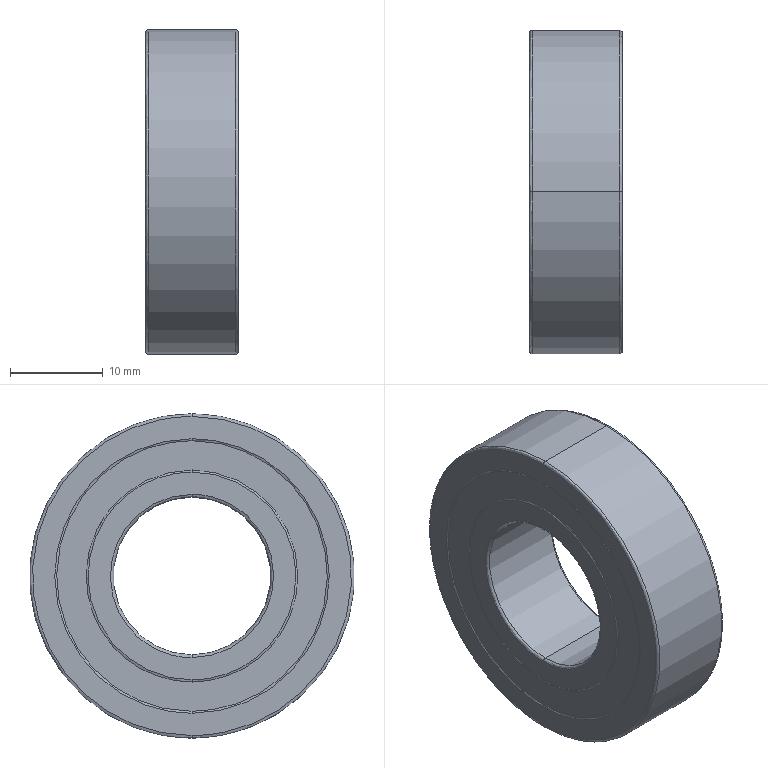Part | SolidWorks | features BaseBody 17 | 17 solids | 196 faces | box 10 x 35 x 35 mm | volume 5537 mm3 | spline 89 | cylinder 69 | plane 38 | commonest cylinder face diameters 26.9 x29 25.1 x28 23 x4 29 x4 17 x2 35 x2